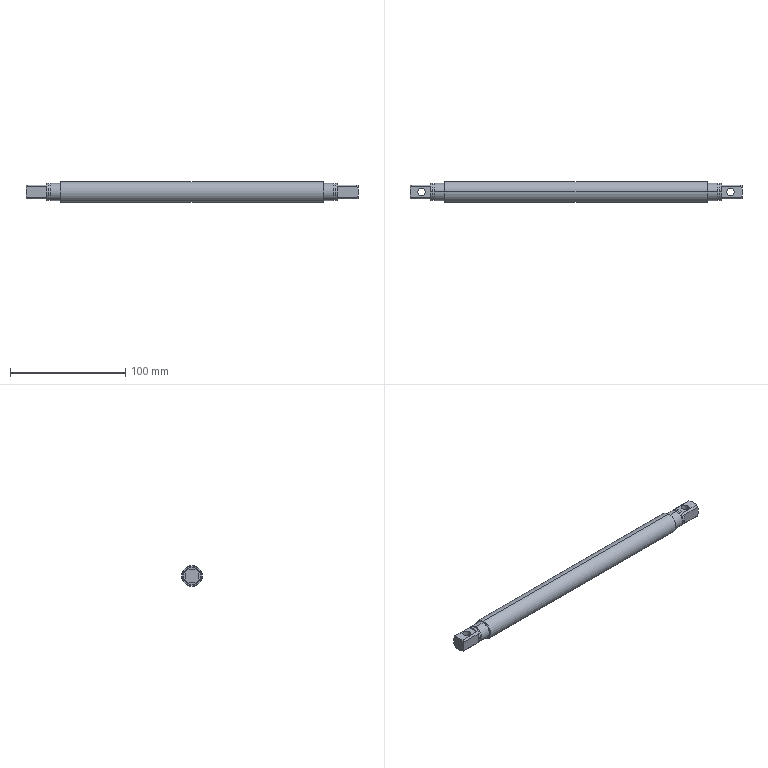Part | STEP file | 1 solid | 54 faces | box 288 x 18 x 18 mm | volume 66372 mm3 | plane 24 | cylinder 18 | cone 12 | commonest cylinder face diameters 15 x8 6.8 x4 14.3 x4 18 x2